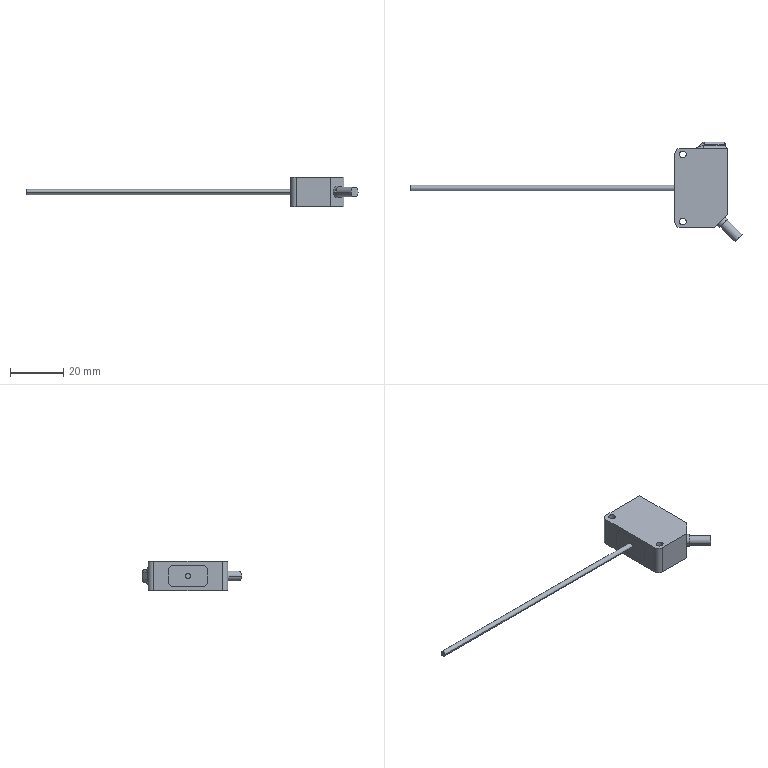Part | SolidWorks | features BaseBody 1 | 1 solid | 64 faces | box 125.214 x 37.614 x 11.2 mm | volume 6967 mm3 | plane 34 | cylinder 26 | sphere 2 | spline 2 | commonest cylinder face diameters 2 x12 4 x6 2.5 x4 3.7 x2 4.5 x2